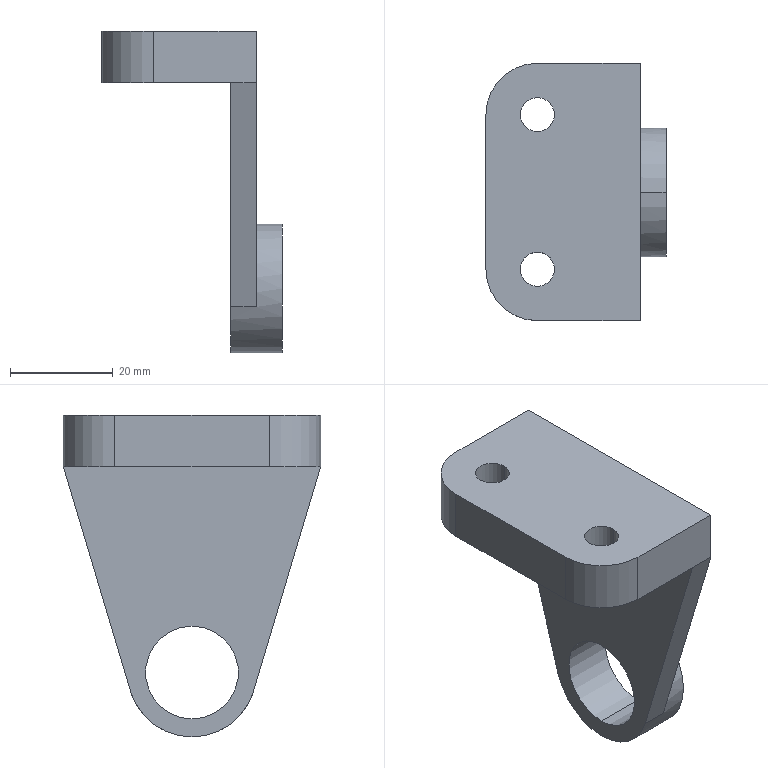Part | SolidWorks | features ICE 3, 3DProfileFeature 1, Extrusion 1, Fillet 1, HoleWzd 1 | 1 solid | 26 faces | box 35 x 50 x 62.5 mm | volume 22031 mm3 | cylinder 14 | plane 12 | commonest cylinder face diameters 6.6 x4 11 x4 18 x2 20 x2 25 x2
STEP:
#1=CARTESIAN_POINT('',(-1.7,15.,5.));
#2=VERTEX_POINT('',#1);
#3=CARTESIAN_POINT('',(-8.3,15.,5.));
#4=VERTEX_POINT('',#3);
#5=CARTESIAN_POINT('',(-5.,15.,5.));
#6=DIRECTION('',(0.,0.,-1.));
#7=DIRECTION('',(1.,0.,0.));
#8=AXIS2_PLACEMENT_3D('',#5,#6,#7);
#9=CIRCLE('',#8,3.3);
#10=EDGE_CURVE('',#2,#4,#9,.T.);
#11=ORIENTED_EDGE('',*,*,#10,.T.);
#12=CARTESIAN_POINT('',(-8.3,15.,10.));
#13=VERTEX_POINT('',#12);
#14=CARTESIAN_POINT('',(-8.3,15.,-22.));
#15=DIRECTION('',(0.,0.,1.));
#16=VECTOR('',#15,1000.);
#17=LINE('',#14,#16);
#18=EDGE_CURVE('',#4,#13,#17,.T.);
#19=ORIENTED_EDGE('',*,*,#18,.T.);
#20=CARTESIAN_POINT('',(-1.7,15.,10.));
#21=VERTEX_POINT('',#20);
#22=CARTESIAN_POINT('',(-5.,15.,10.));
#23=DIRECTION('',(0.,0.,1.));
#24=DIRECTION('',(-1.,0.,0.));
#25=AXIS2_PLACEMENT_3D('',#22,#23,#24);
#26=CIRCLE('',#25,3.3);
#27=EDGE_CURVE('',#13,#21,#26,.T.);
#28=ORIENTED_EDGE('',*,*,#27,.T.);
#29=CARTESIAN_POINT('',(-1.7,15.,-22.));
#30=DIRECTION('',(0.,0.,1.));
#31=VECTOR('',#30,1000.);
#32=LINE('',#29,#31);
#33=EDGE_CURVE('',#2,#21,#32,.T.);
#34=ORIENTED_EDGE('',*,*,#33,.F.);
#35=EDGE_LOOP('',(#11,#19,#28,#34));
#36=FACE_OUTER_BOUND('',#35,.T.);
#37=CARTESIAN_POINT('',(-5.,15.,-22.));
#38=DIRECTION('',(0.,0.,1.));
#39=DIRECTION('',(1.,0.,0.));
#40=AXIS2_PLACEMENT_3D('',#37,#38,#39);
#41=CYLINDRICAL_SURFACE('',#40,3.3);
#42=ADVANCED_FACE('',(#36),#41,.F.);
#43=CARTESIAN_POINT('',(-1.7,-15.,5.));
#44=VERTEX_POINT('',#43);
#45=CARTESIAN_POINT('',(-8.3,-15.,5.));
#46=VERTEX_POINT('',#45);
#47=CARTESIAN_POINT('',(-5.,-15.,5.));
#48=DIRECTION('',(0.,0.,-1.));
#49=DIRECTION('',(1.,0.,0.));
#50=AXIS2_PLACEMENT_3D('',#47,#48,#49);
#51=CIRCLE('',#50,3.3);
#52=EDGE_CURVE('',#44,#46,#51,.T.);
#53=ORIENTED_EDGE('',*,*,#52,.T.);
#54=CARTESIAN_POINT('',(-8.3,-15.,10.));
#55=VERTEX_POINT('',#54);
#56=CARTESIAN_POINT('',(-8.3,-15.,-22.));
#57=DIRECTION('',(0.,0.,1.));
#58=VECTOR('',#57,1000.);
#59=LINE('',#56,#58);
#60=EDGE_CURVE('',#46,#55,#59,.T.);
#61=ORIENTED_EDGE('',*,*,#60,.T.);
#62=CARTESIAN_POINT('',(-1.7,-15.,10.));
#63=VERTEX_POINT('',#62);
#64=CARTESIAN_POINT('',(-5.,-15.,10.));
#65=DIRECTION('',(0.,0.,1.));
#66=DIRECTION('',(-1.,0.,0.));
#67=AXIS2_PLACEMENT_3D('',#64,#65,#66);
#68=CIRCLE('',#67,3.3);
#69=EDGE_CURVE('',#55,#63,#68,.T.);
#70=ORIENTED_EDGE('',*,*,#69,.T.);
#71=CARTESIAN_POINT('',(-1.7,-15.,-22.));
#72=DIRECTION('',(0.,0.,1.));
#73=VECTOR('',#72,1000.);
#74=LINE('',#71,#73);
#75=EDGE_CURVE('',#44,#63,#74,.T.);
#76=ORIENTED_EDGE('',*,*,#75,.F.);
#77=EDGE_LOOP('',(#53,#61,#70,#76));
#78=FACE_OUTER_BOUND('',#77,.T.);
#79=CARTESIAN_POINT('',(-5.,-15.,-22.));
#80=DIRECTION('',(0.,0.,1.));
#81=DIRECTION('',(1.,0.,0.));
#82=AXIS2_PLACEMENT_3D('',#79,#80,#81);
#83=CYLINDRICAL_SURFACE('',#82,3.3);
#84=ADVANCED_FACE('',(#78),#83,.F.);
#85=CARTESIAN_POINT('',(0.5,-15.,5.));
#86=VERTEX_POINT('',#85);
#87=CARTESIAN_POINT('',(-10.5,-15.,5.));
#88=VERTEX_POINT('',#87);
#89=CARTESIAN_POINT('',(-5.,-15.,5.));
#90=DIRECTION('',(0.,0.,-1.));
#91=DIRECTION('',(-1.,0.,0.));
#92=AXIS2_PLACEMENT_3D('',#89,#90,#91);
#93=CIRCLE('',#92,5.5);
#94=EDGE_CURVE('',#86,#88,#93,.T.);
#95=ORIENTED_EDGE('',*,*,#94,.F.);
#96=CARTESIAN_POINT('',(0.5,-15.,0.));
#97=VERTEX_POINT('',#96);
#98=CARTESIAN_POINT('',(0.5,-15.,0.));
#99=DIRECTION('',(0.,0.,-1.));
#100=VECTOR('',#99,1000.);
#101=LINE('',#98,#100);
#102=EDGE_CURVE('',#86,#97,#101,.T.);
#103=ORIENTED_EDGE('',*,*,#102,.T.);
#104=CARTESIAN_POINT('',(-10.5,-15.,0.));
#105=VERTEX_POINT('',#104);
#106=CARTESIAN_POINT('',(-5.,-15.,0.));
#107=DIRECTION('',(0.,0.,-1.));
#108=DIRECTION('',(-1.,0.,0.));
#109=AXIS2_PLACEMENT_3D('',#106,#107,#108);
#110=CIRCLE('',#109,5.5);
#111=EDGE_CURVE('',#97,#105,#110,.T.);
#112=ORIENTED_EDGE('',*,*,#111,.T.);
#113=CARTESIAN_POINT('',(-10.5,-15.,0.));
#114=DIRECTION('',(0.,0.,-1.));
#115=VECTOR('',#114,1000.);
#116=LINE('',#113,#115);
#117=EDGE_CURVE('',#88,#105,#116,.T.);
#118=ORIENTED_EDGE('',*,*,#117,.F.);
#119=EDGE_LOOP('',(#95,#103,#112,#118));
#120=FACE_OUTER_BOUND('',#119,.T.);
#121=CARTESIAN_POINT('',(-5.,-15.,0.));
#122=DIRECTION('',(0.,0.,-1.));
#123=DIRECTION('',(-1.,0.,0.));
#124=AXIS2_PLACEMENT_3D('',#121,#122,#123);
#125=CYLINDRICAL_SURFACE('',#124,5.5);
#126=ADVANCED_FACE('',(#120),#125,.F.);
#127=CARTESIAN_POINT('',(0.5,15.,5.));
#128=VERTEX_POINT('',#127);
#129=CARTESIAN_POINT('',(-10.5,15.,5.));
#130=VERTEX_POINT('',#129);
#131=CARTESIAN_POINT('',(-5.,15.,5.));
#132=DIRECTION('',(0.,0.,-1.));
#133=DIRECTION('',(-1.,0.,0.));
#134=AXIS2_PLACEMENT_3D('',#131,#132,#133);
#135=CIRCLE('',#134,5.5);
#136=EDGE_CURVE('',#128,#130,#135,.T.);
#137=ORIENTED_EDGE('',*,*,#136,.F.);
#138=CARTESIAN_POINT('',(0.5,15.,0.));
#139=VERTEX_POINT('',#138);
#140=CARTESIAN_POINT('',(0.5,15.,0.));
#141=DIRECTION('',(0.,0.,-1.));
#142=VECTOR('',#141,1000.);
#143=LINE('',#140,#142);
#144=EDGE_CURVE('',#128,#139,#143,.T.);
#145=ORIENTED_EDGE('',*,*,#144,.T.);
#146=CARTESIAN_POINT('',(-10.5,15.,0.));
#147=VERTEX_POINT('',#146);
#148=CARTESIAN_POINT('',(-5.,15.,0.));
#149=DIRECTION('',(0.,0.,-1.));
#150=DIRECTION('',(-1.,0.,0.));
#151=AXIS2_PLACEMENT_3D('',#148,#149,#150);
#152=CIRCLE('',#151,5.5);
#153=EDGE_CURVE('',#139,#147,#152,.T.);
#154=ORIENTED_EDGE('',*,*,#153,.T.);
#155=CARTESIAN_POINT('',(-10.5,15.,0.));
#156=DIRECTION('',(0.,0.,-1.));
#157=VECTOR('',#156,1000.);
#158=LINE('',#155,#157);
#159=EDGE_CURVE('',#130,#147,#158,.T.);
#160=ORIENTED_EDGE('',*,*,#159,.F.);
#161=EDGE_LOOP('',(#137,#145,#154,#160));
#162=FACE_OUTER_BOUND('',#161,.T.);
#163=CARTESIAN_POINT('',(-5.,15.,0.));
#164=DIRECTION('',(0.,0.,-1.));
#165=DIRECTION('',(-1.,0.,0.));
#166=AXIS2_PLACEMENT_3D('',#163,#164,#165);
#167=CYLINDRICAL_SURFACE('',#166,5.5);
#168=ADVANCED_FACE('',(#162),#167,.F.);
#169=CARTESIAN_POINT('',(10.,0.,-49.));
#170=VERTEX_POINT('',#169);
#171=CARTESIAN_POINT('',(10.,0.,-31.));
#172=VERTEX_POINT('',#171);
#173=CARTESIAN_POINT('',(10.,0.,-40.));
#174=DIRECTION('',(-1.,0.,0.));
#175=DIRECTION('',(0.,0.,1.));
#176=AXIS2_PLACEMENT_3D('',#173,#174,#175);
#177=CIRCLE('',#176,9.);
#178=EDGE_CURVE('',#170,#172,#177,.T.);
#179=ORIENTED_EDGE('',*,*,#178,.T.);
#180=CARTESIAN_POINT('',(20.,0.,-31.));
#181=VERTEX_POINT('',#180);
#182=CARTESIAN_POINT('',(10.,0.,-31.));
#183=DIRECTION('',(1.,0.,0.));
#184=VECTOR('',#183,1000.);
#185=LINE('',#182,#184);
#186=EDGE_CURVE('',#172,#181,#185,.T.);
#187=ORIENTED_EDGE('',*,*,#186,.T.);
#188=CARTESIAN_POINT('',(20.,0.,-49.));
#189=VERTEX_POINT('',#188);
#190=CARTESIAN_POINT('',(20.,0.,-40.));
#191=DIRECTION('',(1.,0.,0.));
#192=DIRECTION('',(0.,0.,-1.));
#193=AXIS2_PLACEMENT_3D('',#190,#191,#192);
#194=CIRCLE('',#193,9.);
#195=EDGE_CURVE('',#181,#189,#194,.T.);
#196=ORIENTED_EDGE('',*,*,#195,.T.);
#197=CARTESIAN_POINT('',(10.,0.,-49.));
#198=DIRECTION('',(1.,0.,0.));
#199=VECTOR('',#198,1000.);
#200=LINE('',#197,#199);
#201=EDGE_CURVE('',#170,#189,#200,.T.);
#202=ORIENTED_EDGE('',*,*,#201,.F.);
#203=EDGE_LOOP('',(#179,#187,#196,#202));
#204=FACE_OUTER_BOUND('',#203,.T.);
#205=CARTESIAN_POINT('',(10.,0.,-40.));
#206=DIRECTION('',(1.,0.,0.));
#207=DIRECTION('',(0.,0.,-1.));
#208=AXIS2_PLACEMENT_3D('',#205,#206,#207);
#209=CYLINDRICAL_SURFACE('',#208,9.);
#210=ADVANCED_FACE('',(#204),#209,.F.);
#211=CARTESIAN_POINT('',(15.,11.977,-43.579));
#212=VERTEX_POINT('',#211);
#213=CARTESIAN_POINT('',(15.,0.,-27.5));
#214=VERTEX_POINT('',#213);
#215=CARTESIAN_POINT('',(15.,0.,-40.));
#216=DIRECTION('',(1.,0.,0.));
#217=DIRECTION('',(0.,0.,-1.));
#218=AXIS2_PLACEMENT_3D('',#215,#216,#217);
#219=CIRCLE('',#218,12.5);
#220=EDGE_CURVE('',#212,#214,#219,.T.);
#221=ORIENTED_EDGE('',*,*,#220,.T.);
#222=CARTESIAN_POINT('',(20.,0.,-27.5));
#223=VERTEX_POINT('',#222);
#224=CARTESIAN_POINT('',(10.,0.,-27.5));
#225=DIRECTION('',(1.,0.,0.));
#226=VECTOR('',#225,1000.);
#227=LINE('',#224,#226);
#228=EDGE_CURVE('',#214,#223,#227,.T.);
#229=ORIENTED_EDGE('',*,*,#228,.T.);
#230=CARTESIAN_POINT('',(20.,0.,-52.5));
#231=VERTEX_POINT('',#230);
#232=CARTESIAN_POINT('',(20.,0.,-40.));
#233=DIRECTION('',(1.,0.,0.));
#234=DIRECTION('',(0.,0.,-1.));
#235=AXIS2_PLACEMENT_3D('',#232,#233,#234);
#236=CIRCLE('',#235,12.5);
#237=EDGE_CURVE('',#231,#223,#236,.T.);
#238=ORIENTED_EDGE('',*,*,#237,.F.);
#239=CARTESIAN_POINT('',(10.,0.,-52.5));
#240=VERTEX_POINT('',#239);
#241=CARTESIAN_POINT('',(10.,0.,-52.5));
#242=DIRECTION('',(1.,0.,0.));
#243=VECTOR('',#242,1000.);
#244=LINE('',#241,#243);
#245=EDGE_CURVE('',#240,#231,#244,.T.);
#246=ORIENTED_EDGE('',*,*,#245,.F.);
#247=CARTESIAN_POINT('',(10.,11.977,-43.579));
#248=VERTEX_POINT('',#247);
#249=CARTESIAN_POINT('',(10.,0.,-40.));
#250=DIRECTION('',(-1.,0.,0.));
#251=DIRECTION('',(0.,0.,1.));
#252=AXIS2_PLACEMENT_3D('',#249,#250,#251);
#253=CIRCLE('',#252,12.5);
#254=EDGE_CURVE('',#248,#240,#253,.T.);
#255=ORIENTED_EDGE('',*,*,#254,.F.);
#256=CARTESIAN_POINT('',(10.,11.977,-43.579));
#257=DIRECTION('',(1.,0.,0.));
#258=VECTOR('',#257,1000.);
#259=LINE('',#256,#258);
#260=EDGE_CURVE('',#248,#212,#259,.T.);
#261=ORIENTED_EDGE('',*,*,#260,.T.);
#262=EDGE_LOOP('',(#221,#229,#238,#246,#255,#261));
#263=FACE_OUTER_BOUND('',#262,.T.);
#264=CARTESIAN_POINT('',(10.,0.,-40.));
#265=DIRECTION('',(1.,0.,0.));
#266=DIRECTION('',(0.,0.,-1.));
#267=AXIS2_PLACEMENT_3D('',#264,#265,#266);
#268=CYLINDRICAL_SURFACE('',#267,12.5);
#269=ADVANCED_FACE('',(#263),#268,.T.);
#270=ORIENTED_EDGE('',*,*,#220,.F.);
#271=CARTESIAN_POINT('',(15.,25.,0.));
#272=VERTEX_POINT('',#271);
#273=CARTESIAN_POINT('',(15.,11.977,-43.579));
#274=DIRECTION('',(0.,-0.2863,-0.9581));
#275=VECTOR('',#274,1000.);
#276=LINE('',#273,#275);
#277=EDGE_CURVE('',#272,#212,#276,.T.);
#278=ORIENTED_EDGE('',*,*,#277,.F.);
#279=CARTESIAN_POINT('',(15.,25.,10.));
#280=VERTEX_POINT('',#279);
#281=CARTESIAN_POINT('',(15.,25.,10.));
#282=DIRECTION('',(0.,0.,-1.));
#283=VECTOR('',#282,1000.);
#284=LINE('',#281,#283);
#285=EDGE_CURVE('',#280,#272,#284,.T.);
#286=ORIENTED_EDGE('',*,*,#285,.F.);
#287=CARTESIAN_POINT('',(15.,-25.,10.));
#288=VERTEX_POINT('',#287);
#289=CARTESIAN_POINT('',(15.,-25.,10.));
#290=DIRECTION('',(0.,1.,0.));
#291=VECTOR('',#290,1000.);
#292=LINE('',#289,#291);
#293=EDGE_CURVE('',#288,#280,#292,.T.);
#294=ORIENTED_EDGE('',*,*,#293,.F.);
#295=CARTESIAN_POINT('',(15.,-25.,0.));
#296=VERTEX_POINT('',#295);
#297=CARTESIAN_POINT('',(15.,-25.,10.));
#298=DIRECTION('',(0.,0.,-1.));
#299=VECTOR('',#298,1000.);
#300=LINE('',#297,#299);
#301=EDGE_CURVE('',#288,#296,#300,.T.);
#302=ORIENTED_EDGE('',*,*,#301,.T.);
#303=CARTESIAN_POINT('',(15.,-11.977,-43.579));
#304=VERTEX_POINT('',#303);
#305=CARTESIAN_POINT('',(15.,-11.977,-43.579));
#306=DIRECTION('',(0.,-0.2863,0.9581));
#307=VECTOR('',#306,1000.);
#308=LINE('',#305,#307);
#309=EDGE_CURVE('',#304,#296,#308,.T.);
#310=ORIENTED_EDGE('',*,*,#309,.F.);
#311=CARTESIAN_POINT('',(15.,0.,-40.));
#312=DIRECTION('',(1.,0.,0.));
#313=DIRECTION('',(0.,0.,-1.));
#314=AXIS2_PLACEMENT_3D('',#311,#312,#313);
#315=CIRCLE('',#314,12.5);
#316=EDGE_CURVE('',#214,#304,#315,.T.);
#317=ORIENTED_EDGE('',*,*,#316,.F.);
#318=EDGE_LOOP('',(#270,#278,#286,#294,#302,#310,#317));
#319=FACE_OUTER_BOUND('',#318,.T.);
#320=CARTESIAN_POINT('',(15.,-25.,10.));
#321=DIRECTION('',(-1.,0.,0.));
#322=DIRECTION('',(0.,0.,1.));
#323=AXIS2_PLACEMENT_3D('',#320,#321,#322);
#324=PLANE('',#323);
#325=ADVANCED_FACE('',(#319),#324,.F.);
#326=CARTESIAN_POINT('',(10.,25.,0.));
#327=VERTEX_POINT('',#326);
#328=CARTESIAN_POINT('',(-5.,25.,0.));
#329=VERTEX_POINT('',#328);
#330=CARTESIAN_POINT('',(-15.,25.,0.));
#331=DIRECTION('',(-1.,0.,0.));
#332=VECTOR('',#331,1000.);
#333=LINE('',#330,#332);
#334=EDGE_CURVE('',#327,#329,#333,.T.);
#335=ORIENTED_EDGE('',*,*,#334,.T.);
#336=CARTESIAN_POINT('',(-5.,25.,10.));
#337=VERTEX_POINT('',#336);
#338=CARTESIAN_POINT('',(-5.,25.,10.));
#339=DIRECTION('',(0.,0.,1.));
#340=VECTOR('',#339,1000.);
#341=LINE('',#338,#340);
#342=EDGE_CURVE('',#329,#337,#341,.T.);
#343=ORIENTED_EDGE('',*,*,#342,.T.);
#344=CARTESIAN_POINT('',(-15.,25.,10.));
#345=DIRECTION('',(-1.,0.,0.));
#346=VECTOR('',#345,1000.);
#347=LINE('',#344,#346);
#348=EDGE_CURVE('',#280,#337,#347,.T.);
#349=ORIENTED_EDGE('',*,*,#348,.F.);
#350=ORIENTED_EDGE('',*,*,#285,.T.);
#351=CARTESIAN_POINT('',(-15.,25.,0.));
#352=DIRECTION('',(-1.,0.,0.));
#353=VECTOR('',#352,1000.);
#354=LINE('',#351,#353);
#355=EDGE_CURVE('',#272,#327,#354,.T.);
#356=ORIENTED_EDGE('',*,*,#355,.T.);
#357=EDGE_LOOP('',(#335,#343,#349,#350,#356));
#358=FACE_OUTER_BOUND('',#357,.T.);
#359=CARTESIAN_POINT('',(-15.,25.,10.));
#360=DIRECTION('',(0.,-1.,0.));
#361=DIRECTION('',(0.,0.,-1.));
#362=AXIS2_PLACEMENT_3D('',#359,#360,#361);
#363=PLANE('',#362);
#364=ADVANCED_FACE('',(#358),#363,.F.);
#365=CARTESIAN_POINT('',(-15.,15.,10.));
#366=VERTEX_POINT('',#365);
#367=CARTESIAN_POINT('',(-15.,-15.,10.));
#368=VERTEX_POINT('',#367);
#369=CARTESIAN_POINT('',(-15.,-25.,10.));
#370=DIRECTION('',(0.,-1.,0.));
#371=VECTOR('',#370,1000.);
#372=LINE('',#369,#371);
#373=EDGE_CURVE('',#366,#368,#372,.T.);
#374=ORIENTED_EDGE('',*,*,#373,.F.);
#375=CARTESIAN_POINT('',(-15.,15.,0.));
#376=VERTEX_POINT('',#375);
#377=CARTESIAN_POINT('',(-15.,15.,10.));
#378=DIRECTION('',(0.,0.,-1.));
#379=VECTOR('',#378,1000.);
#380=LINE('',#377,#379);
#381=EDGE_CURVE('',#366,#376,#380,.T.);
#382=ORIENTED_EDGE('',*,*,#381,.T.);
#383=CARTESIAN_POINT('',(-15.,-15.,0.));
#384=VERTEX_POINT('',#383);
#385=CARTESIAN_POINT('',(-15.,-25.,0.));
#386=DIRECTION('',(0.,-1.,0.));
#387=VECTOR('',#386,1000.);
#388=LINE('',#385,#387);
#389=EDGE_CURVE('',#376,#384,#388,.T.);
#390=ORIENTED_EDGE('',*,*,#389,.T.);
#391=CARTESIAN_POINT('',(-15.,-15.,10.));
#392=DIRECTION('',(0.,0.,1.));
#393=VECTOR('',#392,1000.);
#394=LINE('',#391,#393);
#395=EDGE_CURVE('',#384,#368,#394,.T.);
#396=ORIENTED_EDGE('',*,*,#395,.T.);
#397=EDGE_LOOP('',(#374,#382,#390,#396));
#398=FACE_OUTER_BOUND('',#397,.T.);
#399=CARTESIAN_POINT('',(-15.,-25.,10.));
#400=DIRECTION('',(1.,0.,0.));
#401=DIRECTION('',(0.,0.,-1.));
#402=AXIS2_PLACEMENT_3D('',#399,#400,#401);
#403=PLANE('',#402);
#404=ADVANCED_FACE('',(#398),#403,.F.);
#405=CARTESIAN_POINT('',(-5.,-25.,10.));
#406=VERTEX_POINT('',#405);
#407=CARTESIAN_POINT('',(-15.,-25.,10.));
#408=DIRECTION('',(1.,0.,0.));
#409=VECTOR('',#408,1000.);
#410=LINE('',#407,#409);
#411=EDGE_CURVE('',#406,#288,#410,.T.);
#412=ORIENTED_EDGE('',*,*,#411,.F.);
#413=CARTESIAN_POINT('',(-5.,-25.,0.));
#414=VERTEX_POINT('',#413);
#415=CARTESIAN_POINT('',(-5.,-25.,10.));
#416=DIRECTION('',(0.,0.,-1.));
#417=VECTOR('',#416,1000.);
#418=LINE('',#415,#417);
#419=EDGE_CURVE('',#406,#414,#418,.T.);
#420=ORIENTED_EDGE('',*,*,#419,.T.);
#421=CARTESIAN_POINT('',(10.,-25.,0.));
#422=VERTEX_POINT('',#421);
#423=CARTESIAN_POINT('',(-15.,-25.,0.));
#424=DIRECTION('',(1.,0.,0.));
#425=VECTOR('',#424,1000.);
#426=LINE('',#423,#425);
#427=EDGE_CURVE('',#414,#422,#426,.T.);
#428=ORIENTED_EDGE('',*,*,#427,.T.);
#429=CARTESIAN_POINT('',(10.,-25.,0.));
#430=DIRECTION('',(1.,0.,0.));
#431=VECTOR('',#430,1000.);
#432=LINE('',#429,#431);
#433=EDGE_CURVE('',#422,#296,#432,.T.);
#434=ORIENTED_EDGE('',*,*,#433,.T.);
#435=ORIENTED_EDGE('',*,*,#301,.F.);
#436=EDGE_LOOP('',(#412,#420,#428,#434,#435));
#437=FACE_OUTER_BOUND('',#436,.T.);
#438=CARTESIAN_POINT('',(-15.,-25.,10.));
#439=DIRECTION('',(0.,1.,0.));
#440=DIRECTION('',(0.,0.,1.));
#441=AXIS2_PLACEMENT_3D('',#438,#439,#440);
#442=PLANE('',#441);
#443=ADVANCED_FACE('',(#437),#442,.F.);
#444=CARTESIAN_POINT('',(-5.,-15.,10.));
#445=DIRECTION('',(0.,0.,1.));
#446=DIRECTION('',(-1.,0.,0.));
#447=AXIS2_PLACEMENT_3D('',#444,#445,#446);
#448=CIRCLE('',#447,3.3);
#449=EDGE_CURVE('',#63,#55,#448,.T.);
#450=ORIENTED_EDGE('',*,*,#449,.F.);
#451=ORIENTED_EDGE('',*,*,#69,.F.);
#452=EDGE_LOOP('',(#450,#451));
#453=FACE_BOUND('',#452,.T.);
#454=CARTESIAN_POINT('',(-5.,15.,10.));
#455=DIRECTION('',(0.,0.,1.));
#456=DIRECTION('',(-1.,0.,0.));
#457=AXIS2_PLACEMENT_3D('',#454,#455,#456);
#458=CIRCLE('',#457,3.3);
#459=EDGE_CURVE('',#21,#13,#458,.T.);
#460=ORIENTED_EDGE('',*,*,#459,.F.);
#461=ORIENTED_EDGE('',*,*,#27,.F.);
#462=EDGE_LOOP('',(#460,#461));
#463=FACE_BOUND('',#462,.T.);
#464=ORIENTED_EDGE('',*,*,#348,.T.);
#465=CARTESIAN_POINT('',(-5.,15.,10.));
#466=DIRECTION('',(0.,0.,1.));
#467=DIRECTION('',(-1.,0.,0.));
#468=AXIS2_PLACEMENT_3D('',#465,#466,#467);
#469=CIRCLE('',#468,10.);
#470=EDGE_CURVE('',#337,#366,#469,.T.);
#471=ORIENTED_EDGE('',*,*,#470,.T.);
#472=ORIENTED_EDGE('',*,*,#373,.T.);
#473=CARTESIAN_POINT('',(-5.,-15.,10.));
#474=DIRECTION('',(0.,0.,1.));
#475=DIRECTION('',(-1.,0.,0.));
#476=AXIS2_PLACEMENT_3D('',#473,#474,#475);
#477=CIRCLE('',#476,10.);
#478=EDGE_CURVE('',#368,#406,#477,.T.);
#479=ORIENTED_EDGE('',*,*,#478,.T.);
#480=ORIENTED_EDGE('',*,*,#411,.T.);
#481=ORIENTED_EDGE('',*,*,#293,.T.);
#482=EDGE_LOOP('',(#464,#471,#472,#479,#480,#481));
#483=FACE_OUTER_BOUND('',#482,.T.);
#484=CARTESIAN_POINT('',(0.,0.,10.));
#485=DIRECTION('',(0.,0.,-1.));
#486=DIRECTION('',(-1.,0.,0.));
#487=AXIS2_PLACEMENT_3D('',#484,#485,#486);
#488=PLANE('',#487);
#489=ADVANCED_FACE('',(#453,#463,#483),#488,.F.);
#490=CARTESIAN_POINT('',(-5.,-15.,0.));
#491=DIRECTION('',(0.,0.,-1.));
#492=DIRECTION('',(-1.,0.,0.));
#493=AXIS2_PLACEMENT_3D('',#490,#491,#492);
#494=CIRCLE('',#493,5.5);
#495=EDGE_CURVE('',#105,#97,#494,.T.);
#496=ORIENTED_EDGE('',*,*,#495,.F.);
#497=ORIENTED_EDGE('',*,*,#111,.F.);
#498=EDGE_LOOP('',(#496,#497));
#499=FACE_BOUND('',#498,.T.);
#500=CARTESIAN_POINT('',(-5.,15.,0.));
#501=DIRECTION('',(0.,0.,-1.));
#502=DIRECTION('',(-1.,0.,0.));
#503=AXIS2_PLACEMENT_3D('',#500,#501,#502);
#504=CIRCLE('',#503,5.5);
#505=EDGE_CURVE('',#147,#139,#504,.T.);
#506=ORIENTED_EDGE('',*,*,#505,.F.);
#507=ORIENTED_EDGE('',*,*,#153,.F.);
#508=EDGE_LOOP('',(#506,#507));
#509=FACE_BOUND('',#508,.T.);
#510=ORIENTED_EDGE('',*,*,#389,.F.);
#511=CARTESIAN_POINT('',(-5.,15.,0.));
#512=DIRECTION('',(0.,0.,-1.));
#513=DIRECTION('',(-1.,0.,0.));
#514=AXIS2_PLACEMENT_3D('',#511,#512,#513);
#515=CIRCLE('',#514,10.);
#516=EDGE_CURVE('',#376,#329,#515,.T.);
#517=ORIENTED_EDGE('',*,*,#516,.T.);
#518=ORIENTED_EDGE('',*,*,#334,.F.);
#519=CARTESIAN_POINT('',(10.,-25.,0.));
#520=DIRECTION('',(0.,1.,0.));
#521=VECTOR('',#520,1000.);
#522=LINE('',#519,#521);
#523=EDGE_CURVE('',#422,#327,#522,.T.);
#524=ORIENTED_EDGE('',*,*,#523,.F.);
#525=ORIENTED_EDGE('',*,*,#427,.F.);
#526=CARTESIAN_POINT('',(-5.,-15.,0.));
#527=DIRECTION('',(0.,0.,-1.));
#528=DIRECTION('',(-1.,0.,0.));
#529=AXIS2_PLACEMENT_3D('',#526,#527,#528);
#530=CIRCLE('',#529,10.);
#531=EDGE_CURVE('',#414,#384,#530,.T.);
#532=ORIENTED_EDGE('',*,*,#531,.T.);
#533=EDGE_LOOP('',(#510,#517,#518,#524,#525,#532));
#534=FACE_OUTER_BOUND('',#533,.T.);
#535=CARTESIAN_POINT('',(0.,0.,0.));
#536=DIRECTION('',(0.,0.,-1.));
#537=DIRECTION('',(-1.,0.,0.));
#538=AXIS2_PLACEMENT_3D('',#535,#536,#537);
#539=PLANE('',#538);
#540=ADVANCED_FACE('',(#499,#509,#534),#539,.T.);
#541=ORIENTED_EDGE('',*,*,#254,.T.);
#542=CARTESIAN_POINT('',(10.,-11.977,-43.579));
#543=VERTEX_POINT('',#542);
#544=CARTESIAN_POINT('',(10.,0.,-40.));
#545=DIRECTION('',(-1.,0.,0.));
#546=DIRECTION('',(0.,0.,1.));
#547=AXIS2_PLACEMENT_3D('',#544,#545,#546);
#548=CIRCLE('',#547,12.5);
#549=EDGE_CURVE('',#240,#543,#548,.T.);
#550=ORIENTED_EDGE('',*,*,#549,.T.);
#551=CARTESIAN_POINT('',(10.,-11.977,-43.579));
#552=DIRECTION('',(0.,-0.2863,0.9581));
#553=VECTOR('',#552,1000.);
#554=LINE('',#551,#553);
#555=EDGE_CURVE('',#543,#422,#554,.T.);
#556=ORIENTED_EDGE('',*,*,#555,.T.);
#557=ORIENTED_EDGE('',*,*,#523,.T.);
#558=CARTESIAN_POINT('',(10.,11.977,-43.579));
#559=DIRECTION('',(0.,-0.2863,-0.9581));
#560=VECTOR('',#559,1000.);
#561=LINE('',#558,#560);
#562=EDGE_CURVE('',#327,#248,#561,.T.);
#563=ORIENTED_EDGE('',*,*,#562,.T.);
#564=EDGE_LOOP('',(#541,#550,#556,#557,#563));
#565=FACE_OUTER_BOUND('',#564,.T.);
#566=ORIENTED_EDGE('',*,*,#178,.F.);
#567=CARTESIAN_POINT('',(10.,0.,-40.));
#568=DIRECTION('',(-1.,0.,0.));
#569=DIRECTION('',(0.,0.,1.));
#570=AXIS2_PLACEMENT_3D('',#567,#568,#569);
#571=CIRCLE('',#570,9.);
#572=EDGE_CURVE('',#172,#170,#571,.T.);
#573=ORIENTED_EDGE('',*,*,#572,.F.);
#574=EDGE_LOOP('',(#566,#573));
#575=FACE_BOUND('',#574,.T.);
#576=CARTESIAN_POINT('',(10.,0.,-40.));
#577=DIRECTION('',(-1.,0.,0.));
#578=DIRECTION('',(0.,0.,1.));
#579=AXIS2_PLACEMENT_3D('',#576,#577,#578);
#580=PLANE('',#579);
#581=ADVANCED_FACE('',(#565,#575),#580,.T.);
#582=ORIENTED_EDGE('',*,*,#228,.F.);
#583=ORIENTED_EDGE('',*,*,#316,.T.);
#584=CARTESIAN_POINT('',(10.,-11.977,-43.579));
#585=DIRECTION('',(1.,0.,0.));
#586=VECTOR('',#585,1000.);
#587=LINE('',#584,#586);
#588=EDGE_CURVE('',#543,#304,#587,.T.);
#589=ORIENTED_EDGE('',*,*,#588,.F.);
#590=ORIENTED_EDGE('',*,*,#549,.F.);
#591=ORIENTED_EDGE('',*,*,#245,.T.);
#592=CARTESIAN_POINT('',(20.,0.,-40.));
#593=DIRECTION('',(1.,0.,0.));
#594=DIRECTION('',(0.,0.,-1.));
#595=AXIS2_PLACEMENT_3D('',#592,#593,#594);
#596=CIRCLE('',#595,12.5);
#597=EDGE_CURVE('',#223,#231,#596,.T.);
#598=ORIENTED_EDGE('',*,*,#597,.F.);
#599=EDGE_LOOP('',(#582,#583,#589,#590,#591,#598));
#600=FACE_OUTER_BOUND('',#599,.T.);
#601=CARTESIAN_POINT('',(10.,0.,-40.));
#602=DIRECTION('',(1.,0.,0.));
#603=DIRECTION('',(0.,0.,-1.));
#604=AXIS2_PLACEMENT_3D('',#601,#602,#603);
#605=CYLINDRICAL_SURFACE('',#604,12.5);
#606=ADVANCED_FACE('',(#600),#605,.T.);
#607=ORIENTED_EDGE('',*,*,#309,.T.);
#608=ORIENTED_EDGE('',*,*,#433,.F.);
#609=ORIENTED_EDGE('',*,*,#555,.F.);
#610=ORIENTED_EDGE('',*,*,#588,.T.);
#611=EDGE_LOOP('',(#607,#608,#609,#610));
#612=FACE_OUTER_BOUND('',#611,.T.);
#613=CARTESIAN_POINT('',(10.,-11.977,-43.579));
#614=DIRECTION('',(0.,0.9581,0.2863));
#615=DIRECTION('',(0.,-0.2863,0.9581));
#616=AXIS2_PLACEMENT_3D('',#613,#614,#615);
#617=PLANE('',#616);
#618=ADVANCED_FACE('',(#612),#617,.F.);
#619=ORIENTED_EDGE('',*,*,#277,.T.);
#620=ORIENTED_EDGE('',*,*,#260,.F.);
#621=ORIENTED_EDGE('',*,*,#562,.F.);
#622=ORIENTED_EDGE('',*,*,#355,.F.);
#623=EDGE_LOOP('',(#619,#620,#621,#622));
#624=FACE_OUTER_BOUND('',#623,.T.);
#625=CARTESIAN_POINT('',(10.,11.977,-43.579));
#626=DIRECTION('',(0.,-0.9581,0.2863));
#627=DIRECTION('',(0.,-0.2863,-0.9581));
#628=AXIS2_PLACEMENT_3D('',#625,#626,#627);
#629=PLANE('',#628);
#630=ADVANCED_FACE('',(#624),#629,.F.);
#631=ORIENTED_EDGE('',*,*,#186,.F.);
#632=ORIENTED_EDGE('',*,*,#572,.T.);
#633=ORIENTED_EDGE('',*,*,#201,.T.);
#634=CARTESIAN_POINT('',(20.,0.,-40.));
#635=DIRECTION('',(1.,0.,0.));
#636=DIRECTION('',(0.,0.,-1.));
#637=AXIS2_PLACEMENT_3D('',#634,#635,#636);
#638=CIRCLE('',#637,9.);
#639=EDGE_CURVE('',#189,#181,#638,.T.);
#640=ORIENTED_EDGE('',*,*,#639,.T.);
#641=EDGE_LOOP('',(#631,#632,#633,#640));
#642=FACE_OUTER_BOUND('',#641,.T.);
#643=CARTESIAN_POINT('',(10.,0.,-40.));
#644=DIRECTION('',(1.,0.,0.));
#645=DIRECTION('',(0.,0.,-1.));
#646=AXIS2_PLACEMENT_3D('',#643,#644,#645);
#647=CYLINDRICAL_SURFACE('',#646,9.);
#648=ADVANCED_FACE('',(#642),#647,.F.);
#649=ORIENTED_EDGE('',*,*,#237,.T.);
#650=ORIENTED_EDGE('',*,*,#597,.T.);
#651=EDGE_LOOP('',(#649,#650));
#652=FACE_OUTER_BOUND('',#651,.T.);
#653=ORIENTED_EDGE('',*,*,#639,.F.);
#654=ORIENTED_EDGE('',*,*,#195,.F.);
#655=EDGE_LOOP('',(#653,#654));
#656=FACE_BOUND('',#655,.T.);
#657=CARTESIAN_POINT('',(20.,0.,-40.));
#658=DIRECTION('',(1.,0.,0.));
#659=DIRECTION('',(0.,0.,-1.));
#660=AXIS2_PLACEMENT_3D('',#657,#658,#659);
#661=PLANE('',#660);
#662=ADVANCED_FACE('',(#652,#656),#661,.T.);
#663=ORIENTED_EDGE('',*,*,#470,.F.);
#664=ORIENTED_EDGE('',*,*,#342,.F.);
#665=ORIENTED_EDGE('',*,*,#516,.F.);
#666=ORIENTED_EDGE('',*,*,#381,.F.);
#667=EDGE_LOOP('',(#663,#664,#665,#666));
#668=FACE_OUTER_BOUND('',#667,.T.);
#669=CARTESIAN_POINT('',(-5.,15.,10.));
#670=DIRECTION('',(0.,0.,-1.));
#671=DIRECTION('',(-1.,0.,0.));
#672=AXIS2_PLACEMENT_3D('',#669,#670,#671);
#673=CYLINDRICAL_SURFACE('',#672,10.);
#674=ADVANCED_FACE('',(#668),#673,.T.);
#675=ORIENTED_EDGE('',*,*,#478,.F.);
#676=ORIENTED_EDGE('',*,*,#395,.F.);
#677=ORIENTED_EDGE('',*,*,#531,.F.);
#678=ORIENTED_EDGE('',*,*,#419,.F.);
#679=EDGE_LOOP('',(#675,#676,#677,#678));
#680=FACE_OUTER_BOUND('',#679,.T.);
#681=CARTESIAN_POINT('',(-5.,-15.,10.));
#682=DIRECTION('',(0.,0.,-1.));
#683=DIRECTION('',(-1.,0.,0.));
#684=AXIS2_PLACEMENT_3D('',#681,#682,#683);
#685=CYLINDRICAL_SURFACE('',#684,10.);
#686=ADVANCED_FACE('',(#680),#685,.T.);
#687=ORIENTED_EDGE('',*,*,#10,.F.);
#688=CARTESIAN_POINT('',(-5.,15.,5.));
#689=DIRECTION('',(0.,0.,-1.));
#690=DIRECTION('',(1.,0.,0.));
#691=AXIS2_PLACEMENT_3D('',#688,#689,#690);
#692=CIRCLE('',#691,3.3);
#693=EDGE_CURVE('',#4,#2,#692,.T.);
#694=ORIENTED_EDGE('',*,*,#693,.F.);
#695=EDGE_LOOP('',(#687,#694));
#696=FACE_BOUND('',#695,.T.);
#697=CARTESIAN_POINT('',(-5.,15.,5.));
#698=DIRECTION('',(0.,0.,-1.));
#699=DIRECTION('',(-1.,0.,0.));
#700=AXIS2_PLACEMENT_3D('',#697,#698,#699);
#701=CIRCLE('',#700,5.5);
#702=EDGE_CURVE('',#130,#128,#701,.T.);
#703=ORIENTED_EDGE('',*,*,#702,.T.);
#704=ORIENTED_EDGE('',*,*,#136,.T.);
#705=EDGE_LOOP('',(#703,#704));
#706=FACE_OUTER_BOUND('',#705,.T.);
#707=CARTESIAN_POINT('',(-1.7,15.,5.));
#708=DIRECTION('',(0.,0.,1.));
#709=DIRECTION('',(1.,0.,0.));
#710=AXIS2_PLACEMENT_3D('',#707,#708,#709);
#711=PLANE('',#710);
#712=ADVANCED_FACE('',(#696,#706),#711,.F.);
#713=ORIENTED_EDGE('',*,*,#144,.F.);
#714=ORIENTED_EDGE('',*,*,#702,.F.);
#715=ORIENTED_EDGE('',*,*,#159,.T.);
#716=ORIENTED_EDGE('',*,*,#505,.T.);
#717=EDGE_LOOP('',(#713,#714,#715,#716));
#718=FACE_OUTER_BOUND('',#717,.T.);
#719=CARTESIAN_POINT('',(-5.,15.,0.));
#720=DIRECTION('',(0.,0.,-1.));
#721=DIRECTION('',(-1.,0.,0.));
#722=AXIS2_PLACEMENT_3D('',#719,#720,#721);
#723=CYLINDRICAL_SURFACE('',#722,5.5);
#724=ADVANCED_FACE('',(#718),#723,.F.);
#725=ORIENTED_EDGE('',*,*,#52,.F.);
#726=CARTESIAN_POINT('',(-5.,-15.,5.));
#727=DIRECTION('',(0.,0.,-1.));
#728=DIRECTION('',(1.,0.,0.));
#729=AXIS2_PLACEMENT_3D('',#726,#727,#728);
#730=CIRCLE('',#729,3.3);
#731=EDGE_CURVE('',#46,#44,#730,.T.);
#732=ORIENTED_EDGE('',*,*,#731,.F.);
#733=EDGE_LOOP('',(#725,#732));
#734=FACE_BOUND('',#733,.T.);
#735=CARTESIAN_POINT('',(-5.,-15.,5.));
#736=DIRECTION('',(0.,0.,-1.));
#737=DIRECTION('',(-1.,0.,0.));
#738=AXIS2_PLACEMENT_3D('',#735,#736,#737);
#739=CIRCLE('',#738,5.5);
#740=EDGE_CURVE('',#88,#86,#739,.T.);
#741=ORIENTED_EDGE('',*,*,#740,.T.);
#742=ORIENTED_EDGE('',*,*,#94,.T.);
#743=EDGE_LOOP('',(#741,#742));
#744=FACE_OUTER_BOUND('',#743,.T.);
#745=CARTESIAN_POINT('',(-1.7,-15.,5.));
#746=DIRECTION('',(0.,0.,1.));
#747=DIRECTION('',(1.,0.,0.));
#748=AXIS2_PLACEMENT_3D('',#745,#746,#747);
#749=PLANE('',#748);
#750=ADVANCED_FACE('',(#734,#744),#749,.F.);
#751=ORIENTED_EDGE('',*,*,#102,.F.);
#752=ORIENTED_EDGE('',*,*,#740,.F.);
#753=ORIENTED_EDGE('',*,*,#117,.T.);
#754=ORIENTED_EDGE('',*,*,#495,.T.);
#755=EDGE_LOOP('',(#751,#752,#753,#754));
#756=FACE_OUTER_BOUND('',#755,.T.);
#757=CARTESIAN_POINT('',(-5.,-15.,0.));
#758=DIRECTION('',(0.,0.,-1.));
#759=DIRECTION('',(-1.,0.,0.));
#760=AXIS2_PLACEMENT_3D('',#757,#758,#759);
#761=CYLINDRICAL_SURFACE('',#760,5.5);
#762=ADVANCED_FACE('',(#756),#761,.F.);
#763=ORIENTED_EDGE('',*,*,#60,.F.);
#764=ORIENTED_EDGE('',*,*,#731,.T.);
#765=ORIENTED_EDGE('',*,*,#75,.T.);
#766=ORIENTED_EDGE('',*,*,#449,.T.);
#767=EDGE_LOOP('',(#763,#764,#765,#766));
#768=FACE_OUTER_BOUND('',#767,.T.);
#769=CARTESIAN_POINT('',(-5.,-15.,-22.));
#770=DIRECTION('',(0.,0.,1.));
#771=DIRECTION('',(1.,0.,0.));
#772=AXIS2_PLACEMENT_3D('',#769,#770,#771);
#773=CYLINDRICAL_SURFACE('',#772,3.3);
#774=ADVANCED_FACE('',(#768),#773,.F.);
#775=ORIENTED_EDGE('',*,*,#18,.F.);
#776=ORIENTED_EDGE('',*,*,#693,.T.);
#777=ORIENTED_EDGE('',*,*,#33,.T.);
#778=ORIENTED_EDGE('',*,*,#459,.T.);
#779=EDGE_LOOP('',(#775,#776,#777,#778));
#780=FACE_OUTER_BOUND('',#779,.T.);
#781=CARTESIAN_POINT('',(-5.,15.,-22.));
#782=DIRECTION('',(0.,0.,1.));
#783=DIRECTION('',(1.,0.,0.));
#784=AXIS2_PLACEMENT_3D('',#781,#782,#783);
#785=CYLINDRICAL_SURFACE('',#784,3.3);
#786=ADVANCED_FACE('',(#780),#785,.F.);
#787=CLOSED_SHELL('',(#42,#84,#126,#168,#210,#269,#325,#364,#404,#443,#489,#540,#581,#606,#618,#630,#648,#662,#674,#686,#712,#724,#750,#762,#774,#786));
#788=MANIFOLD_SOLID_BREP('',#787);
#789=CARTESIAN_POINT('',(0.,0.,0.));
#790=DIRECTION('',(0.,0.,1.));
#791=DIRECTION('',(1.,0.,0.));
#792=AXIS2_PLACEMENT_3D('',#789,#790,#791);
#793=(LENGTH_UNIT()NAMED_UNIT(*)SI_UNIT(.MILLI.,.METRE.));
#794=UNCERTAINTY_MEASURE_WITH_UNIT(LENGTH_MEASURE(0.00001),#793,'','');
#795=(NAMED_UNIT(*)PLANE_ANGLE_UNIT()SI_UNIT($,.RADIAN.));
#796=(NAMED_UNIT(*)SI_UNIT($,.STERADIAN.)SOLID_ANGLE_UNIT());
#797=(GEOMETRIC_REPRESENTATION_CONTEXT(3)GLOBAL_UNCERTAINTY_ASSIGNED_CONTEXT((#794))GLOBAL_UNIT_ASSIGNED_CONTEXT((#793,#795,#796))REPRESENTATION_CONTEXT('',''));
#798=ADVANCED_BREP_SHAPE_REPRESENTATION('',(#788,#792),#797);